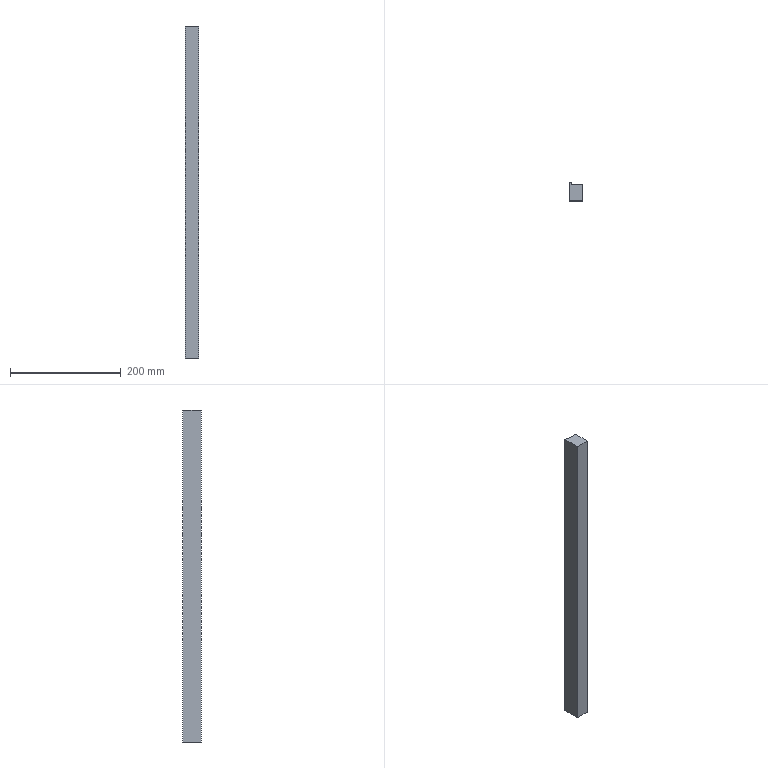Part | SolidWorks | features Extrusion 1 | 1 solid | 8 faces | box 25 x 33 x 600 mm | volume 457200 mm3 | plane 8
STEP:
#1=CARTESIAN_POINT('',(-10.,-12.5,-900.));
#2=VERTEX_POINT('',#1);
#3=CARTESIAN_POINT('',(-10.,-15.5,-900.));
#4=VERTEX_POINT('',#3);
#5=CARTESIAN_POINT('',(-10.,-15.5,-900.));
#6=DIRECTION('',(0.,-1.,0.));
#7=VECTOR('',#6,1000.);
#8=LINE('',#5,#7);
#9=EDGE_CURVE('',#2,#4,#8,.T.);
#10=ORIENTED_EDGE('',*,*,#9,.F.);
#11=CARTESIAN_POINT('',(-10.,-12.5,-300.));
#12=VERTEX_POINT('',#11);
#13=CARTESIAN_POINT('',(-10.,-12.5,-941.4));
#14=DIRECTION('',(0.,0.,1.));
#15=VECTOR('',#14,1000.);
#16=LINE('',#13,#15);
#17=EDGE_CURVE('',#2,#12,#16,.T.);
#18=ORIENTED_EDGE('',*,*,#17,.T.);
#19=CARTESIAN_POINT('',(-10.,-15.5,-300.));
#20=VERTEX_POINT('',#19);
#21=CARTESIAN_POINT('',(-10.,-15.5,-300.));
#22=DIRECTION('',(0.,1.,0.));
#23=VECTOR('',#22,1000.);
#24=LINE('',#21,#23);
#25=EDGE_CURVE('',#20,#12,#24,.T.);
#26=ORIENTED_EDGE('',*,*,#25,.F.);
#27=CARTESIAN_POINT('',(-10.,-15.5,-941.4));
#28=DIRECTION('',(0.,0.,1.));
#29=VECTOR('',#28,1000.);
#30=LINE('',#27,#29);
#31=EDGE_CURVE('',#4,#20,#30,.T.);
#32=ORIENTED_EDGE('',*,*,#31,.F.);
#33=EDGE_LOOP('',(#10,#18,#26,#32));
#34=FACE_OUTER_BOUND('',#33,.T.);
#35=CARTESIAN_POINT('',(-10.,-15.5,-941.4));
#36=DIRECTION('',(1.,0.,0.));
#37=DIRECTION('',(0.,0.,-1.));
#38=AXIS2_PLACEMENT_3D('',#35,#36,#37);
#39=PLANE('',#38);
#40=ADVANCED_FACE('',(#34),#39,.T.);
#41=CARTESIAN_POINT('',(11.,-15.5,-900.));
#42=VERTEX_POINT('',#41);
#43=CARTESIAN_POINT('',(11.,-15.5,-900.));
#44=DIRECTION('',(1.,0.,0.));
#45=VECTOR('',#44,1000.);
#46=LINE('',#43,#45);
#47=EDGE_CURVE('',#4,#42,#46,.T.);
#48=ORIENTED_EDGE('',*,*,#47,.F.);
#49=ORIENTED_EDGE('',*,*,#31,.T.);
#50=CARTESIAN_POINT('',(11.,-15.5,-300.));
#51=VERTEX_POINT('',#50);
#52=CARTESIAN_POINT('',(11.,-15.5,-300.));
#53=DIRECTION('',(-1.,0.,0.));
#54=VECTOR('',#53,1000.);
#55=LINE('',#52,#54);
#56=EDGE_CURVE('',#51,#20,#55,.T.);
#57=ORIENTED_EDGE('',*,*,#56,.F.);
#58=CARTESIAN_POINT('',(11.,-15.5,-941.4));
#59=DIRECTION('',(0.,0.,1.));
#60=VECTOR('',#59,1000.);
#61=LINE('',#58,#60);
#62=EDGE_CURVE('',#42,#51,#61,.T.);
#63=ORIENTED_EDGE('',*,*,#62,.F.);
#64=EDGE_LOOP('',(#48,#49,#57,#63));
#65=FACE_OUTER_BOUND('',#64,.T.);
#66=CARTESIAN_POINT('',(11.,-15.5,-941.4));
#67=DIRECTION('',(0.,1.,0.));
#68=DIRECTION('',(-1.,0.,0.));
#69=AXIS2_PLACEMENT_3D('',#66,#67,#68);
#70=PLANE('',#69);
#71=ADVANCED_FACE('',(#65),#70,.T.);
#72=CARTESIAN_POINT('',(11.,-45.5,-900.));
#73=VERTEX_POINT('',#72);
#74=CARTESIAN_POINT('',(11.,-45.5,-900.));
#75=DIRECTION('',(0.,-1.,0.));
#76=VECTOR('',#75,1000.);
#77=LINE('',#74,#76);
#78=EDGE_CURVE('',#42,#73,#77,.T.);
#79=ORIENTED_EDGE('',*,*,#78,.F.);
#80=ORIENTED_EDGE('',*,*,#62,.T.);
#81=CARTESIAN_POINT('',(11.,-45.5,-300.));
#82=VERTEX_POINT('',#81);
#83=CARTESIAN_POINT('',(11.,-45.5,-300.));
#84=DIRECTION('',(0.,1.,0.));
#85=VECTOR('',#84,1000.);
#86=LINE('',#83,#85);
#87=EDGE_CURVE('',#82,#51,#86,.T.);
#88=ORIENTED_EDGE('',*,*,#87,.F.);
#89=CARTESIAN_POINT('',(11.,-45.5,-941.4));
#90=DIRECTION('',(0.,0.,1.));
#91=VECTOR('',#90,1000.);
#92=LINE('',#89,#91);
#93=EDGE_CURVE('',#73,#82,#92,.T.);
#94=ORIENTED_EDGE('',*,*,#93,.F.);
#95=EDGE_LOOP('',(#79,#80,#88,#94));
#96=FACE_OUTER_BOUND('',#95,.T.);
#97=CARTESIAN_POINT('',(11.,-45.5,-941.4));
#98=DIRECTION('',(1.,0.,0.));
#99=DIRECTION('',(0.,0.,-1.));
#100=AXIS2_PLACEMENT_3D('',#97,#98,#99);
#101=PLANE('',#100);
#102=ADVANCED_FACE('',(#96),#101,.T.);
#103=CARTESIAN_POINT('',(-14.,-45.5,-900.));
#104=VERTEX_POINT('',#103);
#105=CARTESIAN_POINT('',(-14.,-45.5,-900.));
#106=DIRECTION('',(-1.,0.,0.));
#107=VECTOR('',#106,1000.);
#108=LINE('',#105,#107);
#109=EDGE_CURVE('',#73,#104,#108,.T.);
#110=ORIENTED_EDGE('',*,*,#109,.F.);
#111=ORIENTED_EDGE('',*,*,#93,.T.);
#112=CARTESIAN_POINT('',(-14.,-45.5,-300.));
#113=VERTEX_POINT('',#112);
#114=CARTESIAN_POINT('',(-14.,-45.5,-300.));
#115=DIRECTION('',(1.,0.,0.));
#116=VECTOR('',#115,1000.);
#117=LINE('',#114,#116);
#118=EDGE_CURVE('',#113,#82,#117,.T.);
#119=ORIENTED_EDGE('',*,*,#118,.F.);
#120=CARTESIAN_POINT('',(-14.,-45.5,-941.4));
#121=DIRECTION('',(0.,0.,1.));
#122=VECTOR('',#121,1000.);
#123=LINE('',#120,#122);
#124=EDGE_CURVE('',#104,#113,#123,.T.);
#125=ORIENTED_EDGE('',*,*,#124,.F.);
#126=EDGE_LOOP('',(#110,#111,#119,#125));
#127=FACE_OUTER_BOUND('',#126,.T.);
#128=CARTESIAN_POINT('',(-14.,-45.5,-941.4));
#129=DIRECTION('',(0.,-1.,0.));
#130=DIRECTION('',(0.,0.,-1.));
#131=AXIS2_PLACEMENT_3D('',#128,#129,#130);
#132=PLANE('',#131);
#133=ADVANCED_FACE('',(#127),#132,.T.);
#134=CARTESIAN_POINT('',(-14.,-12.5,-900.));
#135=VERTEX_POINT('',#134);
#136=CARTESIAN_POINT('',(-14.,-12.5,-900.));
#137=DIRECTION('',(0.,1.,0.));
#138=VECTOR('',#137,1000.);
#139=LINE('',#136,#138);
#140=EDGE_CURVE('',#104,#135,#139,.T.);
#141=ORIENTED_EDGE('',*,*,#140,.F.);
#142=ORIENTED_EDGE('',*,*,#124,.T.);
#143=CARTESIAN_POINT('',(-14.,-12.5,-300.));
#144=VERTEX_POINT('',#143);
#145=CARTESIAN_POINT('',(-14.,-12.5,-300.));
#146=DIRECTION('',(0.,-1.,0.));
#147=VECTOR('',#146,1000.);
#148=LINE('',#145,#147);
#149=EDGE_CURVE('',#144,#113,#148,.T.);
#150=ORIENTED_EDGE('',*,*,#149,.F.);
#151=CARTESIAN_POINT('',(-14.,-12.5,-941.4));
#152=DIRECTION('',(0.,0.,1.));
#153=VECTOR('',#152,1000.);
#154=LINE('',#151,#153);
#155=EDGE_CURVE('',#135,#144,#154,.T.);
#156=ORIENTED_EDGE('',*,*,#155,.F.);
#157=EDGE_LOOP('',(#141,#142,#150,#156));
#158=FACE_OUTER_BOUND('',#157,.T.);
#159=CARTESIAN_POINT('',(-14.,-12.5,-941.4));
#160=DIRECTION('',(-1.,0.,0.));
#161=DIRECTION('',(0.,-1.,0.));
#162=AXIS2_PLACEMENT_3D('',#159,#160,#161);
#163=PLANE('',#162);
#164=ADVANCED_FACE('',(#158),#163,.T.);
#165=CARTESIAN_POINT('',(-10.,-12.5,-900.));
#166=DIRECTION('',(1.,0.,0.));
#167=VECTOR('',#166,1000.);
#168=LINE('',#165,#167);
#169=EDGE_CURVE('',#135,#2,#168,.T.);
#170=ORIENTED_EDGE('',*,*,#169,.F.);
#171=ORIENTED_EDGE('',*,*,#155,.T.);
#172=CARTESIAN_POINT('',(-10.,-12.5,-300.));
#173=DIRECTION('',(-1.,0.,0.));
#174=VECTOR('',#173,1000.);
#175=LINE('',#172,#174);
#176=EDGE_CURVE('',#12,#144,#175,.T.);
#177=ORIENTED_EDGE('',*,*,#176,.F.);
#178=ORIENTED_EDGE('',*,*,#17,.F.);
#179=EDGE_LOOP('',(#170,#171,#177,#178));
#180=FACE_OUTER_BOUND('',#179,.T.);
#181=CARTESIAN_POINT('',(-10.,-12.5,-941.4));
#182=DIRECTION('',(0.,1.,0.));
#183=DIRECTION('',(0.,0.,1.));
#184=AXIS2_PLACEMENT_3D('',#181,#182,#183);
#185=PLANE('',#184);
#186=ADVANCED_FACE('',(#180),#185,.T.);
#187=ORIENTED_EDGE('',*,*,#25,.T.);
#188=ORIENTED_EDGE('',*,*,#176,.T.);
#189=ORIENTED_EDGE('',*,*,#149,.T.);
#190=ORIENTED_EDGE('',*,*,#118,.T.);
#191=ORIENTED_EDGE('',*,*,#87,.T.);
#192=ORIENTED_EDGE('',*,*,#56,.T.);
#193=EDGE_LOOP('',(#187,#188,#189,#190,#191,#192));
#194=FACE_OUTER_BOUND('',#193,.T.);
#195=CARTESIAN_POINT('',(0.,0.,-300.));
#196=DIRECTION('',(0.,0.,1.));
#197=DIRECTION('',(1.,0.,0.));
#198=AXIS2_PLACEMENT_3D('',#195,#196,#197);
#199=PLANE('',#198);
#200=ADVANCED_FACE('',(#194),#199,.T.);
#201=ORIENTED_EDGE('',*,*,#9,.T.);
#202=ORIENTED_EDGE('',*,*,#47,.T.);
#203=ORIENTED_EDGE('',*,*,#78,.T.);
#204=ORIENTED_EDGE('',*,*,#109,.T.);
#205=ORIENTED_EDGE('',*,*,#140,.T.);
#206=ORIENTED_EDGE('',*,*,#169,.T.);
#207=EDGE_LOOP('',(#201,#202,#203,#204,#205,#206));
#208=FACE_OUTER_BOUND('',#207,.T.);
#209=CARTESIAN_POINT('',(-139.,-44.,-900.));
#210=DIRECTION('',(0.,0.,1.));
#211=DIRECTION('',(0.,-1.,0.));
#212=AXIS2_PLACEMENT_3D('',#209,#210,#211);
#213=PLANE('',#212);
#214=ADVANCED_FACE('',(#208),#213,.F.);
#215=CLOSED_SHELL('',(#40,#71,#102,#133,#164,#186,#200,#214));
#216=MANIFOLD_SOLID_BREP('',#215);
#217=CARTESIAN_POINT('',(0.,0.,0.));
#218=DIRECTION('',(0.,0.,1.));
#219=DIRECTION('',(1.,0.,0.));
#220=AXIS2_PLACEMENT_3D('',#217,#218,#219);
#221=(LENGTH_UNIT()NAMED_UNIT(*)SI_UNIT(.MILLI.,.METRE.));
#222=UNCERTAINTY_MEASURE_WITH_UNIT(LENGTH_MEASURE(0.00001),#221,'','');
#223=(NAMED_UNIT(*)PLANE_ANGLE_UNIT()SI_UNIT($,.RADIAN.));
#224=(NAMED_UNIT(*)SI_UNIT($,.STERADIAN.)SOLID_ANGLE_UNIT());
#225=(GEOMETRIC_REPRESENTATION_CONTEXT(3)GLOBAL_UNCERTAINTY_ASSIGNED_CONTEXT((#222))GLOBAL_UNIT_ASSIGNED_CONTEXT((#221,#223,#224))REPRESENTATION_CONTEXT('',''));
#226=ADVANCED_BREP_SHAPE_REPRESENTATION('',(#216,#220),#225);